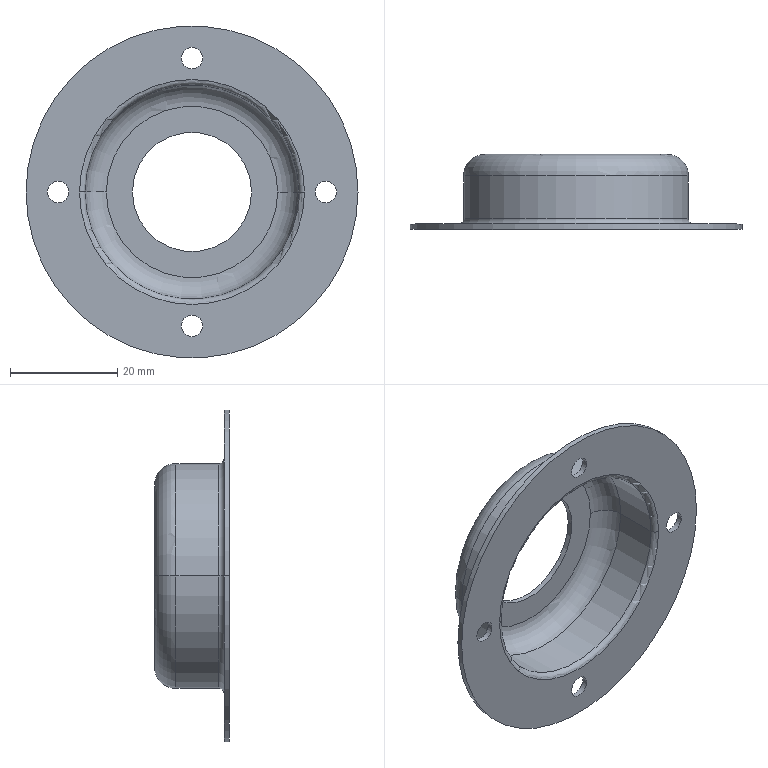Part | SolidWorks | features ICE 2, Revolution 1 | 1 solid | 28 faces | box 62 x 14 x 62 mm | volume 4234 mm3 | cylinder 16 | torus 8 | plane 4 | commonest cylinder face diameters 4 x8 22.26 x2 40 x2 42 x2 62 x2
STEP:
#1=CARTESIAN_POINT('',(-11.13,12.,0.));
#2=VERTEX_POINT('',#1);
#3=CARTESIAN_POINT('',(11.13,12.,0.));
#4=VERTEX_POINT('',#3);
#5=CARTESIAN_POINT('',(0.,12.,0.));
#6=DIRECTION('',(0.,-1.,0.));
#7=DIRECTION('',(1.,0.,0.));
#8=AXIS2_PLACEMENT_3D('',#5,#6,#7);
#9=CIRCLE('',#8,11.13);
#10=EDGE_CURVE('',#2,#4,#9,.T.);
#11=ORIENTED_EDGE('',*,*,#10,.T.);
#12=CARTESIAN_POINT('',(11.13,13.,0.));
#13=VERTEX_POINT('',#12);
#14=CARTESIAN_POINT('',(11.13,3.,0.));
#15=DIRECTION('',(0.,1.,0.));
#16=VECTOR('',#15,1000.);
#17=LINE('',#14,#16);
#18=EDGE_CURVE('',#4,#13,#17,.T.);
#19=ORIENTED_EDGE('',*,*,#18,.T.);
#20=CARTESIAN_POINT('',(-11.13,13.,0.));
#21=VERTEX_POINT('',#20);
#22=CARTESIAN_POINT('',(0.,13.,0.));
#23=DIRECTION('',(0.,1.,0.));
#24=DIRECTION('',(-1.,0.,0.));
#25=AXIS2_PLACEMENT_3D('',#22,#23,#24);
#26=CIRCLE('',#25,11.13);
#27=EDGE_CURVE('',#13,#21,#26,.T.);
#28=ORIENTED_EDGE('',*,*,#27,.T.);
#29=CARTESIAN_POINT('',(-11.13,3.,0.));
#30=DIRECTION('',(0.,1.,0.));
#31=VECTOR('',#30,1000.);
#32=LINE('',#29,#31);
#33=EDGE_CURVE('',#2,#21,#32,.T.);
#34=ORIENTED_EDGE('',*,*,#33,.F.);
#35=EDGE_LOOP('',(#11,#19,#28,#34));
#36=FACE_OUTER_BOUND('',#35,.T.);
#37=CARTESIAN_POINT('',(0.,3.,0.));
#38=DIRECTION('',(0.,1.,0.));
#39=DIRECTION('',(-1.,0.,0.));
#40=AXIS2_PLACEMENT_3D('',#37,#38,#39);
#41=CYLINDRICAL_SURFACE('',#40,11.13);
#42=ADVANCED_FACE('',(#36),#41,.F.);
#43=CARTESIAN_POINT('',(-23.,-1.,0.));
#44=VERTEX_POINT('',#43);
#45=CARTESIAN_POINT('',(-27.,-1.,0.));
#46=VERTEX_POINT('',#45);
#47=CARTESIAN_POINT('',(-25.,-1.,0.));
#48=DIRECTION('',(0.,1.,0.));
#49=DIRECTION('',(1.,0.,0.));
#50=AXIS2_PLACEMENT_3D('',#47,#48,#49);
#51=CIRCLE('',#50,2.);
#52=EDGE_CURVE('',#44,#46,#51,.T.);
#53=ORIENTED_EDGE('',*,*,#52,.F.);
#54=CARTESIAN_POINT('',(-23.,0.,0.));
#55=VERTEX_POINT('',#54);
#56=CARTESIAN_POINT('',(-23.,-6.657,0.));
#57=DIRECTION('',(0.,1.,0.));
#58=VECTOR('',#57,1000.);
#59=LINE('',#56,#58);
#60=EDGE_CURVE('',#44,#55,#59,.T.);
#61=ORIENTED_EDGE('',*,*,#60,.T.);
#62=CARTESIAN_POINT('',(-27.,0.,0.));
#63=VERTEX_POINT('',#62);
#64=CARTESIAN_POINT('',(-25.,0.,0.));
#65=DIRECTION('',(0.,1.,0.));
#66=DIRECTION('',(-1.,0.,0.));
#67=AXIS2_PLACEMENT_3D('',#64,#65,#66);
#68=CIRCLE('',#67,2.);
#69=EDGE_CURVE('',#55,#63,#68,.T.);
#70=ORIENTED_EDGE('',*,*,#69,.T.);
#71=CARTESIAN_POINT('',(-27.,-6.657,0.));
#72=DIRECTION('',(0.,1.,0.));
#73=VECTOR('',#72,1000.);
#74=LINE('',#71,#73);
#75=EDGE_CURVE('',#46,#63,#74,.T.);
#76=ORIENTED_EDGE('',*,*,#75,.F.);
#77=EDGE_LOOP('',(#53,#61,#70,#76));
#78=FACE_OUTER_BOUND('',#77,.T.);
#79=CARTESIAN_POINT('',(-25.,-6.657,0.));
#80=DIRECTION('',(0.,1.,0.));
#81=DIRECTION('',(-1.,0.,0.));
#82=AXIS2_PLACEMENT_3D('',#79,#80,#81);
#83=CYLINDRICAL_SURFACE('',#82,2.);
#84=ADVANCED_FACE('',(#78),#83,.F.);
#85=CARTESIAN_POINT('',(2.,-1.,25.));
#86=VERTEX_POINT('',#85);
#87=CARTESIAN_POINT('',(-2.,-1.,25.));
#88=VERTEX_POINT('',#87);
#89=CARTESIAN_POINT('',(0.,-1.,25.));
#90=DIRECTION('',(0.,1.,0.));
#91=DIRECTION('',(1.,0.,0.));
#92=AXIS2_PLACEMENT_3D('',#89,#90,#91);
#93=CIRCLE('',#92,2.);
#94=EDGE_CURVE('',#86,#88,#93,.T.);
#95=ORIENTED_EDGE('',*,*,#94,.F.);
#96=CARTESIAN_POINT('',(2.,0.,25.));
#97=VERTEX_POINT('',#96);
#98=CARTESIAN_POINT('',(2.,-6.657,25.));
#99=DIRECTION('',(0.,1.,0.));
#100=VECTOR('',#99,1000.);
#101=LINE('',#98,#100);
#102=EDGE_CURVE('',#86,#97,#101,.T.);
#103=ORIENTED_EDGE('',*,*,#102,.T.);
#104=CARTESIAN_POINT('',(-2.,0.,25.));
#105=VERTEX_POINT('',#104);
#106=CARTESIAN_POINT('',(0.,0.,25.));
#107=DIRECTION('',(0.,1.,0.));
#108=DIRECTION('',(-1.,0.,0.));
#109=AXIS2_PLACEMENT_3D('',#106,#107,#108);
#110=CIRCLE('',#109,2.);
#111=EDGE_CURVE('',#97,#105,#110,.T.);
#112=ORIENTED_EDGE('',*,*,#111,.T.);
#113=CARTESIAN_POINT('',(-2.,-6.657,25.));
#114=DIRECTION('',(0.,1.,0.));
#115=VECTOR('',#114,1000.);
#116=LINE('',#113,#115);
#117=EDGE_CURVE('',#88,#105,#116,.T.);
#118=ORIENTED_EDGE('',*,*,#117,.F.);
#119=EDGE_LOOP('',(#95,#103,#112,#118));
#120=FACE_OUTER_BOUND('',#119,.T.);
#121=CARTESIAN_POINT('',(0.,-6.657,25.));
#122=DIRECTION('',(0.,1.,0.));
#123=DIRECTION('',(-1.,0.,0.));
#124=AXIS2_PLACEMENT_3D('',#121,#122,#123);
#125=CYLINDRICAL_SURFACE('',#124,2.);
#126=ADVANCED_FACE('',(#120),#125,.F.);
#127=CARTESIAN_POINT('',(27.,-1.,0.));
#128=VERTEX_POINT('',#127);
#129=CARTESIAN_POINT('',(23.,-1.,0.));
#130=VERTEX_POINT('',#129);
#131=CARTESIAN_POINT('',(25.,-1.,0.));
#132=DIRECTION('',(0.,1.,0.));
#133=DIRECTION('',(1.,0.,0.));
#134=AXIS2_PLACEMENT_3D('',#131,#132,#133);
#135=CIRCLE('',#134,2.);
#136=EDGE_CURVE('',#128,#130,#135,.T.);
#137=ORIENTED_EDGE('',*,*,#136,.F.);
#138=CARTESIAN_POINT('',(27.,0.,0.));
#139=VERTEX_POINT('',#138);
#140=CARTESIAN_POINT('',(27.,-6.657,0.));
#141=DIRECTION('',(0.,1.,0.));
#142=VECTOR('',#141,1000.);
#143=LINE('',#140,#142);
#144=EDGE_CURVE('',#128,#139,#143,.T.);
#145=ORIENTED_EDGE('',*,*,#144,.T.);
#146=CARTESIAN_POINT('',(23.,0.,0.));
#147=VERTEX_POINT('',#146);
#148=CARTESIAN_POINT('',(25.,0.,0.));
#149=DIRECTION('',(0.,1.,0.));
#150=DIRECTION('',(-1.,0.,0.));
#151=AXIS2_PLACEMENT_3D('',#148,#149,#150);
#152=CIRCLE('',#151,2.);
#153=EDGE_CURVE('',#139,#147,#152,.T.);
#154=ORIENTED_EDGE('',*,*,#153,.T.);
#155=CARTESIAN_POINT('',(23.,-6.657,0.));
#156=DIRECTION('',(0.,1.,0.));
#157=VECTOR('',#156,1000.);
#158=LINE('',#155,#157);
#159=EDGE_CURVE('',#130,#147,#158,.T.);
#160=ORIENTED_EDGE('',*,*,#159,.F.);
#161=EDGE_LOOP('',(#137,#145,#154,#160));
#162=FACE_OUTER_BOUND('',#161,.T.);
#163=CARTESIAN_POINT('',(25.,-6.657,0.));
#164=DIRECTION('',(0.,1.,0.));
#165=DIRECTION('',(-1.,0.,0.));
#166=AXIS2_PLACEMENT_3D('',#163,#164,#165);
#167=CYLINDRICAL_SURFACE('',#166,2.);
#168=ADVANCED_FACE('',(#162),#167,.F.);
#169=CARTESIAN_POINT('',(2.,-1.,-25.));
#170=VERTEX_POINT('',#169);
#171=CARTESIAN_POINT('',(-2.,-1.,-25.));
#172=VERTEX_POINT('',#171);
#173=CARTESIAN_POINT('',(0.,-1.,-25.));
#174=DIRECTION('',(0.,1.,0.));
#175=DIRECTION('',(1.,0.,0.));
#176=AXIS2_PLACEMENT_3D('',#173,#174,#175);
#177=CIRCLE('',#176,2.);
#178=EDGE_CURVE('',#170,#172,#177,.T.);
#179=ORIENTED_EDGE('',*,*,#178,.F.);
#180=CARTESIAN_POINT('',(2.,0.,-25.));
#181=VERTEX_POINT('',#180);
#182=CARTESIAN_POINT('',(2.,-6.657,-25.));
#183=DIRECTION('',(0.,1.,0.));
#184=VECTOR('',#183,1000.);
#185=LINE('',#182,#184);
#186=EDGE_CURVE('',#170,#181,#185,.T.);
#187=ORIENTED_EDGE('',*,*,#186,.T.);
#188=CARTESIAN_POINT('',(-2.,0.,-25.));
#189=VERTEX_POINT('',#188);
#190=CARTESIAN_POINT('',(0.,0.,-25.));
#191=DIRECTION('',(0.,1.,0.));
#192=DIRECTION('',(-1.,0.,0.));
#193=AXIS2_PLACEMENT_3D('',#190,#191,#192);
#194=CIRCLE('',#193,2.);
#195=EDGE_CURVE('',#181,#189,#194,.T.);
#196=ORIENTED_EDGE('',*,*,#195,.T.);
#197=CARTESIAN_POINT('',(-2.,-6.657,-25.));
#198=DIRECTION('',(0.,1.,0.));
#199=VECTOR('',#198,1000.);
#200=LINE('',#197,#199);
#201=EDGE_CURVE('',#172,#189,#200,.T.);
#202=ORIENTED_EDGE('',*,*,#201,.F.);
#203=EDGE_LOOP('',(#179,#187,#196,#202));
#204=FACE_OUTER_BOUND('',#203,.T.);
#205=CARTESIAN_POINT('',(0.,-6.657,-25.));
#206=DIRECTION('',(0.,1.,0.));
#207=DIRECTION('',(-1.,0.,0.));
#208=AXIS2_PLACEMENT_3D('',#205,#206,#207);
#209=CYLINDRICAL_SURFACE('',#208,2.);
#210=ADVANCED_FACE('',(#204),#209,.F.);
#211=CARTESIAN_POINT('',(21.,-1.,0.));
#212=VERTEX_POINT('',#211);
#213=CARTESIAN_POINT('',(-21.,-1.,0.));
#214=VERTEX_POINT('',#213);
#215=CARTESIAN_POINT('',(0.,-1.,0.));
#216=DIRECTION('',(0.,-1.,0.));
#217=DIRECTION('',(1.,0.,0.));
#218=AXIS2_PLACEMENT_3D('',#215,#216,#217);
#219=CIRCLE('',#218,21.);
#220=EDGE_CURVE('',#212,#214,#219,.T.);
#221=ORIENTED_EDGE('',*,*,#220,.T.);
#222=CARTESIAN_POINT('',(-20.,0.,0.));
#223=VERTEX_POINT('',#222);
#224=CARTESIAN_POINT('',(-21.,0.,0.));
#225=DIRECTION('',(0.,0.,1.));
#226=DIRECTION('',(1.,0.,0.));
#227=AXIS2_PLACEMENT_3D('',#224,#225,#226);
#228=CIRCLE('',#227,1.);
#229=EDGE_CURVE('',#214,#223,#228,.T.);
#230=ORIENTED_EDGE('',*,*,#229,.T.);
#231=CARTESIAN_POINT('',(20.,0.,0.));
#232=VERTEX_POINT('',#231);
#233=CARTESIAN_POINT('',(0.,0.,0.));
#234=DIRECTION('',(0.,-1.,0.));
#235=DIRECTION('',(1.,0.,0.));
#236=AXIS2_PLACEMENT_3D('',#233,#234,#235);
#237=CIRCLE('',#236,20.);
#238=EDGE_CURVE('',#232,#223,#237,.T.);
#239=ORIENTED_EDGE('',*,*,#238,.F.);
#240=CARTESIAN_POINT('',(21.,0.,0.));
#241=DIRECTION('',(0.,0.,-1.));
#242=DIRECTION('',(-1.,0.,0.));
#243=AXIS2_PLACEMENT_3D('',#240,#241,#242);
#244=CIRCLE('',#243,1.);
#245=EDGE_CURVE('',#212,#232,#244,.T.);
#246=ORIENTED_EDGE('',*,*,#245,.F.);
#247=EDGE_LOOP('',(#221,#230,#239,#246));
#248=FACE_OUTER_BOUND('',#247,.T.);
#249=CARTESIAN_POINT('',(0.,0.,0.));
#250=DIRECTION('',(0.,-1.,0.));
#251=DIRECTION('',(1.,0.,0.));
#252=AXIS2_PLACEMENT_3D('',#249,#250,#251);
#253=TOROIDAL_SURFACE('',#252,21.,1.);
#254=ADVANCED_FACE('',(#248),#253,.T.);
#255=CARTESIAN_POINT('',(-20.,8.,0.));
#256=VERTEX_POINT('',#255);
#257=CARTESIAN_POINT('',(20.,8.,0.));
#258=VERTEX_POINT('',#257);
#259=CARTESIAN_POINT('',(0.,8.,0.));
#260=DIRECTION('',(0.,-1.,0.));
#261=DIRECTION('',(1.,0.,0.));
#262=AXIS2_PLACEMENT_3D('',#259,#260,#261);
#263=CIRCLE('',#262,20.);
#264=EDGE_CURVE('',#256,#258,#263,.T.);
#265=ORIENTED_EDGE('',*,*,#264,.F.);
#266=CARTESIAN_POINT('',(-20.,0.,0.));
#267=DIRECTION('',(0.,-1.,0.));
#268=VECTOR('',#267,1000.);
#269=LINE('',#266,#268);
#270=EDGE_CURVE('',#256,#223,#269,.T.);
#271=ORIENTED_EDGE('',*,*,#270,.T.);
#272=CARTESIAN_POINT('',(0.,0.,0.));
#273=DIRECTION('',(0.,-1.,0.));
#274=DIRECTION('',(1.,0.,0.));
#275=AXIS2_PLACEMENT_3D('',#272,#273,#274);
#276=CIRCLE('',#275,20.);
#277=EDGE_CURVE('',#223,#232,#276,.T.);
#278=ORIENTED_EDGE('',*,*,#277,.T.);
#279=CARTESIAN_POINT('',(20.,0.,0.));
#280=DIRECTION('',(0.,-1.,0.));
#281=VECTOR('',#280,1000.);
#282=LINE('',#279,#281);
#283=EDGE_CURVE('',#258,#232,#282,.T.);
#284=ORIENTED_EDGE('',*,*,#283,.F.);
#285=EDGE_LOOP('',(#265,#271,#278,#284));
#286=FACE_OUTER_BOUND('',#285,.T.);
#287=CARTESIAN_POINT('',(0.,0.,0.));
#288=DIRECTION('',(0.,-1.,0.));
#289=DIRECTION('',(1.,0.,0.));
#290=AXIS2_PLACEMENT_3D('',#287,#288,#289);
#291=CYLINDRICAL_SURFACE('',#290,20.);
#292=ADVANCED_FACE('',(#286),#291,.F.);
#293=CARTESIAN_POINT('',(-16.,12.,0.));
#294=VERTEX_POINT('',#293);
#295=CARTESIAN_POINT('',(16.,12.,0.));
#296=VERTEX_POINT('',#295);
#297=CARTESIAN_POINT('',(0.,12.,0.));
#298=DIRECTION('',(0.,-1.,0.));
#299=DIRECTION('',(1.,0.,0.));
#300=AXIS2_PLACEMENT_3D('',#297,#298,#299);
#301=CIRCLE('',#300,16.);
#302=EDGE_CURVE('',#294,#296,#301,.T.);
#303=ORIENTED_EDGE('',*,*,#302,.F.);
#304=CARTESIAN_POINT('',(-16.,8.,0.));
#305=DIRECTION('',(0.,0.,1.));
#306=DIRECTION('',(1.,0.,0.));
#307=AXIS2_PLACEMENT_3D('',#304,#305,#306);
#308=CIRCLE('',#307,4.);
#309=EDGE_CURVE('',#294,#256,#308,.T.);
#310=ORIENTED_EDGE('',*,*,#309,.T.);
#311=ORIENTED_EDGE('',*,*,#264,.T.);
#312=CARTESIAN_POINT('',(16.,8.,0.));
#313=DIRECTION('',(0.,0.,-1.));
#314=DIRECTION('',(-1.,0.,0.));
#315=AXIS2_PLACEMENT_3D('',#312,#313,#314);
#316=CIRCLE('',#315,4.);
#317=EDGE_CURVE('',#296,#258,#316,.T.);
#318=ORIENTED_EDGE('',*,*,#317,.F.);
#319=EDGE_LOOP('',(#303,#310,#311,#318));
#320=FACE_OUTER_BOUND('',#319,.T.);
#321=CARTESIAN_POINT('',(0.,8.,0.));
#322=DIRECTION('',(0.,-1.,0.));
#323=DIRECTION('',(1.,0.,0.));
#324=AXIS2_PLACEMENT_3D('',#321,#322,#323);
#325=TOROIDAL_SURFACE('',#324,16.,4.);
#326=ADVANCED_FACE('',(#320),#325,.F.);
#327=CARTESIAN_POINT('',(17.,13.,0.));
#328=VERTEX_POINT('',#327);
#329=CARTESIAN_POINT('',(-17.,13.,0.));
#330=VERTEX_POINT('',#329);
#331=CARTESIAN_POINT('',(0.,13.,0.));
#332=DIRECTION('',(0.,-1.,0.));
#333=DIRECTION('',(1.,0.,0.));
#334=AXIS2_PLACEMENT_3D('',#331,#332,#333);
#335=CIRCLE('',#334,17.);
#336=EDGE_CURVE('',#328,#330,#335,.T.);
#337=ORIENTED_EDGE('',*,*,#336,.T.);
#338=CARTESIAN_POINT('',(-21.,9.,0.));
#339=VERTEX_POINT('',#338);
#340=CARTESIAN_POINT('',(-17.,9.,0.));
#341=DIRECTION('',(0.,0.,1.));
#342=DIRECTION('',(1.,0.,0.));
#343=AXIS2_PLACEMENT_3D('',#340,#341,#342);
#344=CIRCLE('',#343,4.);
#345=EDGE_CURVE('',#330,#339,#344,.T.);
#346=ORIENTED_EDGE('',*,*,#345,.T.);
#347=CARTESIAN_POINT('',(21.,9.,0.));
#348=VERTEX_POINT('',#347);
#349=CARTESIAN_POINT('',(0.,9.,0.));
#350=DIRECTION('',(0.,-1.,0.));
#351=DIRECTION('',(1.,0.,0.));
#352=AXIS2_PLACEMENT_3D('',#349,#350,#351);
#353=CIRCLE('',#352,21.);
#354=EDGE_CURVE('',#348,#339,#353,.T.);
#355=ORIENTED_EDGE('',*,*,#354,.F.);
#356=CARTESIAN_POINT('',(17.,9.,0.));
#357=DIRECTION('',(0.,0.,-1.));
#358=DIRECTION('',(-1.,0.,0.));
#359=AXIS2_PLACEMENT_3D('',#356,#357,#358);
#360=CIRCLE('',#359,4.);
#361=EDGE_CURVE('',#328,#348,#360,.T.);
#362=ORIENTED_EDGE('',*,*,#361,.F.);
#363=EDGE_LOOP('',(#337,#346,#355,#362));
#364=FACE_OUTER_BOUND('',#363,.T.);
#365=CARTESIAN_POINT('',(0.,9.,0.));
#366=DIRECTION('',(0.,-1.,0.));
#367=DIRECTION('',(1.,0.,0.));
#368=AXIS2_PLACEMENT_3D('',#365,#366,#367);
#369=TOROIDAL_SURFACE('',#368,17.,4.);
#370=ADVANCED_FACE('',(#364),#369,.T.);
#371=ORIENTED_EDGE('',*,*,#354,.T.);
#372=CARTESIAN_POINT('',(-21.,1.,0.));
#373=VERTEX_POINT('',#372);
#374=CARTESIAN_POINT('',(-21.,0.,0.));
#375=DIRECTION('',(0.,-1.,0.));
#376=VECTOR('',#375,1000.);
#377=LINE('',#374,#376);
#378=EDGE_CURVE('',#339,#373,#377,.T.);
#379=ORIENTED_EDGE('',*,*,#378,.T.);
#380=CARTESIAN_POINT('',(21.,1.,0.));
#381=VERTEX_POINT('',#380);
#382=CARTESIAN_POINT('',(0.,1.,0.));
#383=DIRECTION('',(0.,-1.,0.));
#384=DIRECTION('',(1.,0.,0.));
#385=AXIS2_PLACEMENT_3D('',#382,#383,#384);
#386=CIRCLE('',#385,21.);
#387=EDGE_CURVE('',#381,#373,#386,.T.);
#388=ORIENTED_EDGE('',*,*,#387,.F.);
#389=CARTESIAN_POINT('',(21.,0.,0.));
#390=DIRECTION('',(0.,-1.,0.));
#391=VECTOR('',#390,1000.);
#392=LINE('',#389,#391);
#393=EDGE_CURVE('',#348,#381,#392,.T.);
#394=ORIENTED_EDGE('',*,*,#393,.F.);
#395=EDGE_LOOP('',(#371,#379,#388,#394));
#396=FACE_OUTER_BOUND('',#395,.T.);
#397=CARTESIAN_POINT('',(0.,0.,0.));
#398=DIRECTION('',(0.,-1.,0.));
#399=DIRECTION('',(1.,0.,0.));
#400=AXIS2_PLACEMENT_3D('',#397,#398,#399);
#401=CYLINDRICAL_SURFACE('',#400,21.);
#402=ADVANCED_FACE('',(#396),#401,.T.);
#403=CARTESIAN_POINT('',(-22.,0.,0.));
#404=VERTEX_POINT('',#403);
#405=CARTESIAN_POINT('',(22.,0.,0.));
#406=VERTEX_POINT('',#405);
#407=CARTESIAN_POINT('',(0.,0.,0.));
#408=DIRECTION('',(0.,-1.,0.));
#409=DIRECTION('',(1.,0.,0.));
#410=AXIS2_PLACEMENT_3D('',#407,#408,#409);
#411=CIRCLE('',#410,22.);
#412=EDGE_CURVE('',#404,#406,#411,.T.);
#413=ORIENTED_EDGE('',*,*,#412,.F.);
#414=CARTESIAN_POINT('',(-22.,1.,0.));
#415=DIRECTION('',(0.,0.,1.));
#416=DIRECTION('',(1.,0.,0.));
#417=AXIS2_PLACEMENT_3D('',#414,#415,#416);
#418=CIRCLE('',#417,1.);
#419=EDGE_CURVE('',#404,#373,#418,.T.);
#420=ORIENTED_EDGE('',*,*,#419,.T.);
#421=CARTESIAN_POINT('',(0.,1.,0.));
#422=DIRECTION('',(0.,-1.,0.));
#423=DIRECTION('',(1.,0.,0.));
#424=AXIS2_PLACEMENT_3D('',#421,#422,#423);
#425=CIRCLE('',#424,21.);
#426=EDGE_CURVE('',#373,#381,#425,.T.);
#427=ORIENTED_EDGE('',*,*,#426,.T.);
#428=CARTESIAN_POINT('',(22.,1.,0.));
#429=DIRECTION('',(0.,0.,-1.));
#430=DIRECTION('',(-1.,0.,0.));
#431=AXIS2_PLACEMENT_3D('',#428,#429,#430);
#432=CIRCLE('',#431,1.);
#433=EDGE_CURVE('',#406,#381,#432,.T.);
#434=ORIENTED_EDGE('',*,*,#433,.F.);
#435=EDGE_LOOP('',(#413,#420,#427,#434));
#436=FACE_OUTER_BOUND('',#435,.T.);
#437=CARTESIAN_POINT('',(0.,1.,0.));
#438=DIRECTION('',(0.,-1.,0.));
#439=DIRECTION('',(1.,0.,0.));
#440=AXIS2_PLACEMENT_3D('',#437,#438,#439);
#441=TOROIDAL_SURFACE('',#440,22.,1.);
#442=ADVANCED_FACE('',(#436),#441,.F.);
#443=CARTESIAN_POINT('',(31.,0.,0.));
#444=VERTEX_POINT('',#443);
#445=CARTESIAN_POINT('',(-31.,0.,0.));
#446=VERTEX_POINT('',#445);
#447=CARTESIAN_POINT('',(0.,0.,0.));
#448=DIRECTION('',(0.,-1.,0.));
#449=DIRECTION('',(1.,0.,0.));
#450=AXIS2_PLACEMENT_3D('',#447,#448,#449);
#451=CIRCLE('',#450,31.);
#452=EDGE_CURVE('',#444,#446,#451,.T.);
#453=ORIENTED_EDGE('',*,*,#452,.T.);
#454=CARTESIAN_POINT('',(-31.,-1.,0.));
#455=VERTEX_POINT('',#454);
#456=CARTESIAN_POINT('',(-31.,0.,0.));
#457=DIRECTION('',(0.,-1.,0.));
#458=VECTOR('',#457,1000.);
#459=LINE('',#456,#458);
#460=EDGE_CURVE('',#446,#455,#459,.T.);
#461=ORIENTED_EDGE('',*,*,#460,.T.);
#462=CARTESIAN_POINT('',(31.,-1.,0.));
#463=VERTEX_POINT('',#462);
#464=CARTESIAN_POINT('',(0.,-1.,0.));
#465=DIRECTION('',(0.,-1.,0.));
#466=DIRECTION('',(1.,0.,0.));
#467=AXIS2_PLACEMENT_3D('',#464,#465,#466);
#468=CIRCLE('',#467,31.);
#469=EDGE_CURVE('',#463,#455,#468,.T.);
#470=ORIENTED_EDGE('',*,*,#469,.F.);
#471=CARTESIAN_POINT('',(31.,0.,0.));
#472=DIRECTION('',(0.,-1.,0.));
#473=VECTOR('',#472,1000.);
#474=LINE('',#471,#473);
#475=EDGE_CURVE('',#444,#463,#474,.T.);
#476=ORIENTED_EDGE('',*,*,#475,.F.);
#477=EDGE_LOOP('',(#453,#461,#470,#476));
#478=FACE_OUTER_BOUND('',#477,.T.);
#479=CARTESIAN_POINT('',(0.,0.,0.));
#480=DIRECTION('',(0.,-1.,0.));
#481=DIRECTION('',(1.,0.,0.));
#482=AXIS2_PLACEMENT_3D('',#479,#480,#481);
#483=CYLINDRICAL_SURFACE('',#482,31.);
#484=ADVANCED_FACE('',(#478),#483,.T.);
#485=ORIENTED_EDGE('',*,*,#460,.F.);
#486=CARTESIAN_POINT('',(0.,0.,0.));
#487=DIRECTION('',(0.,-1.,0.));
#488=DIRECTION('',(1.,0.,0.));
#489=AXIS2_PLACEMENT_3D('',#486,#487,#488);
#490=CIRCLE('',#489,31.);
#491=EDGE_CURVE('',#446,#444,#490,.T.);
#492=ORIENTED_EDGE('',*,*,#491,.T.);
#493=ORIENTED_EDGE('',*,*,#475,.T.);
#494=CARTESIAN_POINT('',(0.,-1.,0.));
#495=DIRECTION('',(0.,-1.,0.));
#496=DIRECTION('',(1.,0.,0.));
#497=AXIS2_PLACEMENT_3D('',#494,#495,#496);
#498=CIRCLE('',#497,31.);
#499=EDGE_CURVE('',#455,#463,#498,.T.);
#500=ORIENTED_EDGE('',*,*,#499,.F.);
#501=EDGE_LOOP('',(#485,#492,#493,#500));
#502=FACE_OUTER_BOUND('',#501,.T.);
#503=CARTESIAN_POINT('',(0.,0.,0.));
#504=DIRECTION('',(0.,-1.,0.));
#505=DIRECTION('',(1.,0.,0.));
#506=AXIS2_PLACEMENT_3D('',#503,#504,#505);
#507=CYLINDRICAL_SURFACE('',#506,31.);
#508=ADVANCED_FACE('',(#502),#507,.T.);
#509=CARTESIAN_POINT('',(-25.,0.,0.));
#510=DIRECTION('',(0.,1.,0.));
#511=DIRECTION('',(-1.,0.,0.));
#512=AXIS2_PLACEMENT_3D('',#509,#510,#511);
#513=CIRCLE('',#512,2.);
#514=EDGE_CURVE('',#63,#55,#513,.T.);
#515=ORIENTED_EDGE('',*,*,#514,.F.);
#516=ORIENTED_EDGE('',*,*,#69,.F.);
#517=EDGE_LOOP('',(#515,#516));
#518=FACE_BOUND('',#517,.T.);
#519=CARTESIAN_POINT('',(0.,0.,25.));
#520=DIRECTION('',(0.,1.,0.));
#521=DIRECTION('',(-1.,0.,0.));
#522=AXIS2_PLACEMENT_3D('',#519,#520,#521);
#523=CIRCLE('',#522,2.);
#524=EDGE_CURVE('',#105,#97,#523,.T.);
#525=ORIENTED_EDGE('',*,*,#524,.F.);
#526=ORIENTED_EDGE('',*,*,#111,.F.);
#527=EDGE_LOOP('',(#525,#526));
#528=FACE_BOUND('',#527,.T.);
#529=CARTESIAN_POINT('',(25.,0.,0.));
#530=DIRECTION('',(0.,1.,0.));
#531=DIRECTION('',(-1.,0.,0.));
#532=AXIS2_PLACEMENT_3D('',#529,#530,#531);
#533=CIRCLE('',#532,2.);
#534=EDGE_CURVE('',#147,#139,#533,.T.);
#535=ORIENTED_EDGE('',*,*,#534,.F.);
#536=ORIENTED_EDGE('',*,*,#153,.F.);
#537=EDGE_LOOP('',(#535,#536));
#538=FACE_BOUND('',#537,.T.);
#539=CARTESIAN_POINT('',(0.,0.,-25.));
#540=DIRECTION('',(0.,1.,0.));
#541=DIRECTION('',(-1.,0.,0.));
#542=AXIS2_PLACEMENT_3D('',#539,#540,#541);
#543=CIRCLE('',#542,2.);
#544=EDGE_CURVE('',#189,#181,#543,.T.);
#545=ORIENTED_EDGE('',*,*,#544,.F.);
#546=ORIENTED_EDGE('',*,*,#195,.F.);
#547=EDGE_LOOP('',(#545,#546));
#548=FACE_BOUND('',#547,.T.);
#549=CARTESIAN_POINT('',(0.,0.,0.));
#550=DIRECTION('',(0.,-1.,0.));
#551=DIRECTION('',(1.,0.,0.));
#552=AXIS2_PLACEMENT_3D('',#549,#550,#551);
#553=CIRCLE('',#552,22.);
#554=EDGE_CURVE('',#406,#404,#553,.T.);
#555=ORIENTED_EDGE('',*,*,#554,.T.);
#556=ORIENTED_EDGE('',*,*,#412,.T.);
#557=EDGE_LOOP('',(#555,#556));
#558=FACE_BOUND('',#557,.T.);
#559=ORIENTED_EDGE('',*,*,#452,.F.);
#560=ORIENTED_EDGE('',*,*,#491,.F.);
#561=EDGE_LOOP('',(#559,#560));
#562=FACE_OUTER_BOUND('',#561,.T.);
#563=CARTESIAN_POINT('',(22.,0.,0.));
#564=DIRECTION('',(0.,1.,0.));
#565=DIRECTION('',(-1.,0.,0.));
#566=AXIS2_PLACEMENT_3D('',#563,#564,#565);
#567=PLANE('',#566);
#568=ADVANCED_FACE('',(#518,#528,#538,#548,#558,#562),#567,.T.);
#569=ORIENTED_EDGE('',*,*,#419,.F.);
#570=ORIENTED_EDGE('',*,*,#554,.F.);
#571=ORIENTED_EDGE('',*,*,#433,.T.);
#572=ORIENTED_EDGE('',*,*,#387,.T.);
#573=EDGE_LOOP('',(#569,#570,#571,#572));
#574=FACE_OUTER_BOUND('',#573,.T.);
#575=CARTESIAN_POINT('',(0.,1.,0.));
#576=DIRECTION('',(0.,-1.,0.));
#577=DIRECTION('',(1.,0.,0.));
#578=AXIS2_PLACEMENT_3D('',#575,#576,#577);
#579=TOROIDAL_SURFACE('',#578,22.,1.);
#580=ADVANCED_FACE('',(#574),#579,.F.);
#581=ORIENTED_EDGE('',*,*,#378,.F.);
#582=CARTESIAN_POINT('',(0.,9.,0.));
#583=DIRECTION('',(0.,-1.,0.));
#584=DIRECTION('',(1.,0.,0.));
#585=AXIS2_PLACEMENT_3D('',#582,#583,#584);
#586=CIRCLE('',#585,21.);
#587=EDGE_CURVE('',#339,#348,#586,.T.);
#588=ORIENTED_EDGE('',*,*,#587,.T.);
#589=ORIENTED_EDGE('',*,*,#393,.T.);
#590=ORIENTED_EDGE('',*,*,#426,.F.);
#591=EDGE_LOOP('',(#581,#588,#589,#590));
#592=FACE_OUTER_BOUND('',#591,.T.);
#593=CARTESIAN_POINT('',(0.,0.,0.));
#594=DIRECTION('',(0.,-1.,0.));
#595=DIRECTION('',(1.,0.,0.));
#596=AXIS2_PLACEMENT_3D('',#593,#594,#595);
#597=CYLINDRICAL_SURFACE('',#596,21.);
#598=ADVANCED_FACE('',(#592),#597,.T.);
#599=ORIENTED_EDGE('',*,*,#345,.F.);
#600=CARTESIAN_POINT('',(0.,13.,0.));
#601=DIRECTION('',(0.,-1.,0.));
#602=DIRECTION('',(1.,0.,0.));
#603=AXIS2_PLACEMENT_3D('',#600,#601,#602);
#604=CIRCLE('',#603,17.);
#605=EDGE_CURVE('',#330,#328,#604,.T.);
#606=ORIENTED_EDGE('',*,*,#605,.T.);
#607=ORIENTED_EDGE('',*,*,#361,.T.);
#608=ORIENTED_EDGE('',*,*,#587,.F.);
#609=EDGE_LOOP('',(#599,#606,#607,#608));
#610=FACE_OUTER_BOUND('',#609,.T.);
#611=CARTESIAN_POINT('',(0.,9.,0.));
#612=DIRECTION('',(0.,-1.,0.));
#613=DIRECTION('',(1.,0.,0.));
#614=AXIS2_PLACEMENT_3D('',#611,#612,#613);
#615=TOROIDAL_SURFACE('',#614,17.,4.);
#616=ADVANCED_FACE('',(#610),#615,.T.);
#617=CARTESIAN_POINT('',(0.,13.,0.));
#618=DIRECTION('',(0.,1.,0.));
#619=DIRECTION('',(-1.,0.,0.));
#620=AXIS2_PLACEMENT_3D('',#617,#618,#619);
#621=CIRCLE('',#620,11.13);
#622=EDGE_CURVE('',#21,#13,#621,.T.);
#623=ORIENTED_EDGE('',*,*,#622,.F.);
#624=ORIENTED_EDGE('',*,*,#27,.F.);
#625=EDGE_LOOP('',(#623,#624));
#626=FACE_BOUND('',#625,.T.);
#627=ORIENTED_EDGE('',*,*,#336,.F.);
#628=ORIENTED_EDGE('',*,*,#605,.F.);
#629=EDGE_LOOP('',(#627,#628));
#630=FACE_OUTER_BOUND('',#629,.T.);
#631=CARTESIAN_POINT('',(0.,13.,0.));
#632=DIRECTION('',(0.,1.,0.));
#633=DIRECTION('',(-1.,0.,0.));
#634=AXIS2_PLACEMENT_3D('',#631,#632,#633);
#635=PLANE('',#634);
#636=ADVANCED_FACE('',(#626,#630),#635,.T.);
#637=ORIENTED_EDGE('',*,*,#10,.F.);
#638=CARTESIAN_POINT('',(0.,12.,0.));
#639=DIRECTION('',(0.,-1.,0.));
#640=DIRECTION('',(1.,0.,0.));
#641=AXIS2_PLACEMENT_3D('',#638,#639,#640);
#642=CIRCLE('',#641,11.13);
#643=EDGE_CURVE('',#4,#2,#642,.T.);
#644=ORIENTED_EDGE('',*,*,#643,.F.);
#645=EDGE_LOOP('',(#637,#644));
#646=FACE_BOUND('',#645,.T.);
#647=CARTESIAN_POINT('',(0.,12.,0.));
#648=DIRECTION('',(0.,-1.,0.));
#649=DIRECTION('',(1.,0.,0.));
#650=AXIS2_PLACEMENT_3D('',#647,#648,#649);
#651=CIRCLE('',#650,16.);
#652=EDGE_CURVE('',#296,#294,#651,.T.);
#653=ORIENTED_EDGE('',*,*,#652,.T.);
#654=ORIENTED_EDGE('',*,*,#302,.T.);
#655=EDGE_LOOP('',(#653,#654));
#656=FACE_OUTER_BOUND('',#655,.T.);
#657=CARTESIAN_POINT('',(0.,12.,0.));
#658=DIRECTION('',(0.,-1.,0.));
#659=DIRECTION('',(1.,0.,0.));
#660=AXIS2_PLACEMENT_3D('',#657,#658,#659);
#661=PLANE('',#660);
#662=ADVANCED_FACE('',(#646,#656),#661,.T.);
#663=ORIENTED_EDGE('',*,*,#309,.F.);
#664=ORIENTED_EDGE('',*,*,#652,.F.);
#665=ORIENTED_EDGE('',*,*,#317,.T.);
#666=CARTESIAN_POINT('',(0.,8.,0.));
#667=DIRECTION('',(0.,-1.,0.));
#668=DIRECTION('',(1.,0.,0.));
#669=AXIS2_PLACEMENT_3D('',#666,#667,#668);
#670=CIRCLE('',#669,20.);
#671=EDGE_CURVE('',#258,#256,#670,.T.);
#672=ORIENTED_EDGE('',*,*,#671,.T.);
#673=EDGE_LOOP('',(#663,#664,#665,#672));
#674=FACE_OUTER_BOUND('',#673,.T.);
#675=CARTESIAN_POINT('',(0.,8.,0.));
#676=DIRECTION('',(0.,-1.,0.));
#677=DIRECTION('',(1.,0.,0.));
#678=AXIS2_PLACEMENT_3D('',#675,#676,#677);
#679=TOROIDAL_SURFACE('',#678,16.,4.);
#680=ADVANCED_FACE('',(#674),#679,.F.);
#681=ORIENTED_EDGE('',*,*,#270,.F.);
#682=ORIENTED_EDGE('',*,*,#671,.F.);
#683=ORIENTED_EDGE('',*,*,#283,.T.);
#684=ORIENTED_EDGE('',*,*,#238,.T.);
#685=EDGE_LOOP('',(#681,#682,#683,#684));
#686=FACE_OUTER_BOUND('',#685,.T.);
#687=CARTESIAN_POINT('',(0.,0.,0.));
#688=DIRECTION('',(0.,-1.,0.));
#689=DIRECTION('',(1.,0.,0.));
#690=AXIS2_PLACEMENT_3D('',#687,#688,#689);
#691=CYLINDRICAL_SURFACE('',#690,20.);
#692=ADVANCED_FACE('',(#686),#691,.F.);
#693=ORIENTED_EDGE('',*,*,#229,.F.);
#694=CARTESIAN_POINT('',(0.,-1.,0.));
#695=DIRECTION('',(0.,-1.,0.));
#696=DIRECTION('',(1.,0.,0.));
#697=AXIS2_PLACEMENT_3D('',#694,#695,#696);
#698=CIRCLE('',#697,21.);
#699=EDGE_CURVE('',#214,#212,#698,.T.);
#700=ORIENTED_EDGE('',*,*,#699,.T.);
#701=ORIENTED_EDGE('',*,*,#245,.T.);
#702=ORIENTED_EDGE('',*,*,#277,.F.);
#703=EDGE_LOOP('',(#693,#700,#701,#702));
#704=FACE_OUTER_BOUND('',#703,.T.);
#705=CARTESIAN_POINT('',(0.,0.,0.));
#706=DIRECTION('',(0.,-1.,0.));
#707=DIRECTION('',(1.,0.,0.));
#708=AXIS2_PLACEMENT_3D('',#705,#706,#707);
#709=TOROIDAL_SURFACE('',#708,21.,1.);
#710=ADVANCED_FACE('',(#704),#709,.T.);
#711=CARTESIAN_POINT('',(-25.,-1.,0.));
#712=DIRECTION('',(0.,1.,0.));
#713=DIRECTION('',(1.,0.,0.));
#714=AXIS2_PLACEMENT_3D('',#711,#712,#713);
#715=CIRCLE('',#714,2.);
#716=EDGE_CURVE('',#46,#44,#715,.T.);
#717=ORIENTED_EDGE('',*,*,#716,.T.);
#718=ORIENTED_EDGE('',*,*,#52,.T.);
#719=EDGE_LOOP('',(#717,#718));
#720=FACE_BOUND('',#719,.T.);
#721=CARTESIAN_POINT('',(0.,-1.,25.));
#722=DIRECTION('',(0.,1.,0.));
#723=DIRECTION('',(1.,0.,0.));
#724=AXIS2_PLACEMENT_3D('',#721,#722,#723);
#725=CIRCLE('',#724,2.);
#726=EDGE_CURVE('',#88,#86,#725,.T.);
#727=ORIENTED_EDGE('',*,*,#726,.T.);
#728=ORIENTED_EDGE('',*,*,#94,.T.);
#729=EDGE_LOOP('',(#727,#728));
#730=FACE_BOUND('',#729,.T.);
#731=CARTESIAN_POINT('',(25.,-1.,0.));
#732=DIRECTION('',(0.,1.,0.));
#733=DIRECTION('',(1.,0.,0.));
#734=AXIS2_PLACEMENT_3D('',#731,#732,#733);
#735=CIRCLE('',#734,2.);
#736=EDGE_CURVE('',#130,#128,#735,.T.);
#737=ORIENTED_EDGE('',*,*,#736,.T.);
#738=ORIENTED_EDGE('',*,*,#136,.T.);
#739=EDGE_LOOP('',(#737,#738));
#740=FACE_BOUND('',#739,.T.);
#741=CARTESIAN_POINT('',(0.,-1.,-25.));
#742=DIRECTION('',(0.,1.,0.));
#743=DIRECTION('',(1.,0.,0.));
#744=AXIS2_PLACEMENT_3D('',#741,#742,#743);
#745=CIRCLE('',#744,2.);
#746=EDGE_CURVE('',#172,#170,#745,.T.);
#747=ORIENTED_EDGE('',*,*,#746,.T.);
#748=ORIENTED_EDGE('',*,*,#178,.T.);
#749=EDGE_LOOP('',(#747,#748));
#750=FACE_BOUND('',#749,.T.);
#751=ORIENTED_EDGE('',*,*,#469,.T.);
#752=ORIENTED_EDGE('',*,*,#499,.T.);
#753=EDGE_LOOP('',(#751,#752));
#754=FACE_OUTER_BOUND('',#753,.T.);
#755=ORIENTED_EDGE('',*,*,#220,.F.);
#756=ORIENTED_EDGE('',*,*,#699,.F.);
#757=EDGE_LOOP('',(#755,#756));
#758=FACE_BOUND('',#757,.T.);
#759=CARTESIAN_POINT('',(21.,-1.,0.));
#760=DIRECTION('',(0.,-1.,0.));
#761=DIRECTION('',(1.,0.,0.));
#762=AXIS2_PLACEMENT_3D('',#759,#760,#761);
#763=PLANE('',#762);
#764=ADVANCED_FACE('',(#720,#730,#740,#750,#754,#758),#763,.T.);
#765=ORIENTED_EDGE('',*,*,#186,.F.);
#766=ORIENTED_EDGE('',*,*,#746,.F.);
#767=ORIENTED_EDGE('',*,*,#201,.T.);
#768=ORIENTED_EDGE('',*,*,#544,.T.);
#769=EDGE_LOOP('',(#765,#766,#767,#768));
#770=FACE_OUTER_BOUND('',#769,.T.);
#771=CARTESIAN_POINT('',(0.,-6.657,-25.));
#772=DIRECTION('',(0.,1.,0.));
#773=DIRECTION('',(-1.,0.,0.));
#774=AXIS2_PLACEMENT_3D('',#771,#772,#773);
#775=CYLINDRICAL_SURFACE('',#774,2.);
#776=ADVANCED_FACE('',(#770),#775,.F.);
#777=ORIENTED_EDGE('',*,*,#144,.F.);
#778=ORIENTED_EDGE('',*,*,#736,.F.);
#779=ORIENTED_EDGE('',*,*,#159,.T.);
#780=ORIENTED_EDGE('',*,*,#534,.T.);
#781=EDGE_LOOP('',(#777,#778,#779,#780));
#782=FACE_OUTER_BOUND('',#781,.T.);
#783=CARTESIAN_POINT('',(25.,-6.657,0.));
#784=DIRECTION('',(0.,1.,0.));
#785=DIRECTION('',(-1.,0.,0.));
#786=AXIS2_PLACEMENT_3D('',#783,#784,#785);
#787=CYLINDRICAL_SURFACE('',#786,2.);
#788=ADVANCED_FACE('',(#782),#787,.F.);
#789=ORIENTED_EDGE('',*,*,#102,.F.);
#790=ORIENTED_EDGE('',*,*,#726,.F.);
#791=ORIENTED_EDGE('',*,*,#117,.T.);
#792=ORIENTED_EDGE('',*,*,#524,.T.);
#793=EDGE_LOOP('',(#789,#790,#791,#792));
#794=FACE_OUTER_BOUND('',#793,.T.);
#795=CARTESIAN_POINT('',(0.,-6.657,25.));
#796=DIRECTION('',(0.,1.,0.));
#797=DIRECTION('',(-1.,0.,0.));
#798=AXIS2_PLACEMENT_3D('',#795,#796,#797);
#799=CYLINDRICAL_SURFACE('',#798,2.);
#800=ADVANCED_FACE('',(#794),#799,.F.);
#801=ORIENTED_EDGE('',*,*,#60,.F.);
#802=ORIENTED_EDGE('',*,*,#716,.F.);
#803=ORIENTED_EDGE('',*,*,#75,.T.);
#804=ORIENTED_EDGE('',*,*,#514,.T.);
#805=EDGE_LOOP('',(#801,#802,#803,#804));
#806=FACE_OUTER_BOUND('',#805,.T.);
#807=CARTESIAN_POINT('',(-25.,-6.657,0.));
#808=DIRECTION('',(0.,1.,0.));
#809=DIRECTION('',(-1.,0.,0.));
#810=AXIS2_PLACEMENT_3D('',#807,#808,#809);
#811=CYLINDRICAL_SURFACE('',#810,2.);
#812=ADVANCED_FACE('',(#806),#811,.F.);
#813=ORIENTED_EDGE('',*,*,#18,.F.);
#814=ORIENTED_EDGE('',*,*,#643,.T.);
#815=ORIENTED_EDGE('',*,*,#33,.T.);
#816=ORIENTED_EDGE('',*,*,#622,.T.);
#817=EDGE_LOOP('',(#813,#814,#815,#816));
#818=FACE_OUTER_BOUND('',#817,.T.);
#819=CARTESIAN_POINT('',(0.,3.,0.));
#820=DIRECTION('',(0.,1.,0.));
#821=DIRECTION('',(-1.,0.,0.));
#822=AXIS2_PLACEMENT_3D('',#819,#820,#821);
#823=CYLINDRICAL_SURFACE('',#822,11.13);
#824=ADVANCED_FACE('',(#818),#823,.F.);
#825=CLOSED_SHELL('',(#42,#84,#126,#168,#210,#254,#292,#326,#370,#402,#442,#484,#508,#568,#580,#598,#616,#636,#662,#680,#692,#710,#764,#776,#788,#800,#812,#824));
#826=MANIFOLD_SOLID_BREP('',#825);
#827=CARTESIAN_POINT('',(0.,0.,0.));
#828=DIRECTION('',(0.,0.,1.));
#829=DIRECTION('',(1.,0.,0.));
#830=AXIS2_PLACEMENT_3D('',#827,#828,#829);
#831=(LENGTH_UNIT()NAMED_UNIT(*)SI_UNIT(.MILLI.,.METRE.));
#832=UNCERTAINTY_MEASURE_WITH_UNIT(LENGTH_MEASURE(0.00001),#831,'','');
#833=(NAMED_UNIT(*)PLANE_ANGLE_UNIT()SI_UNIT($,.RADIAN.));
#834=(NAMED_UNIT(*)SI_UNIT($,.STERADIAN.)SOLID_ANGLE_UNIT());
#835=(GEOMETRIC_REPRESENTATION_CONTEXT(3)GLOBAL_UNCERTAINTY_ASSIGNED_CONTEXT((#832))GLOBAL_UNIT_ASSIGNED_CONTEXT((#831,#833,#834))REPRESENTATION_CONTEXT('',''));
#836=ADVANCED_BREP_SHAPE_REPRESENTATION('',(#826,#830),#835);